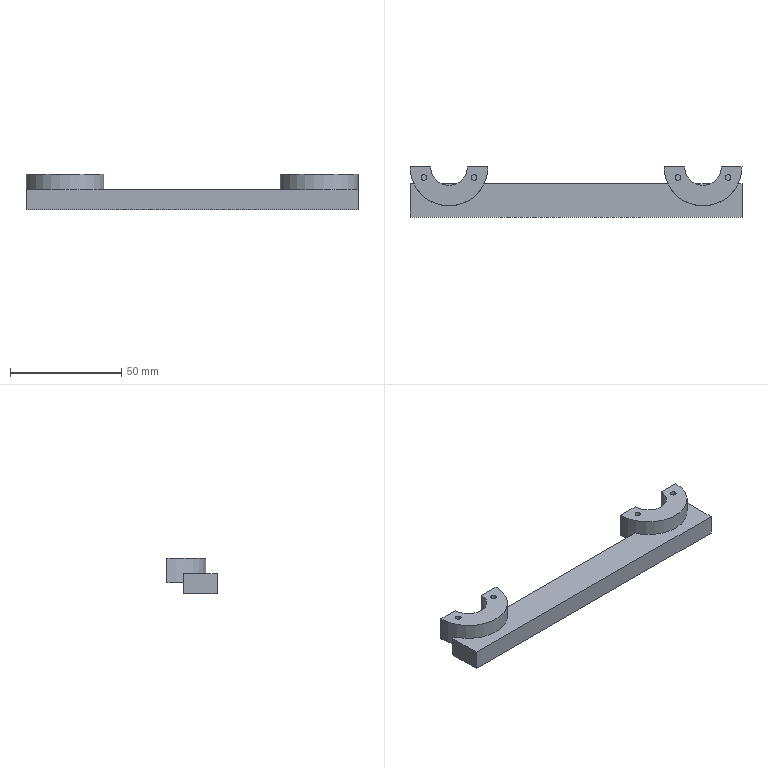NC program | NX | posted with a generic post | part box 149 x 22.5 x 16 mm
Whole program:
N10 G17 G21 G94 G90
(DRILLING , TOOL : ZXZ)
N12 T01 M6
N14 G54
N16 G17 G0 G90 X-68.25 Y4.75 S3000 M3
N18 G43 Z30. H1
N20 G94 G81 G98 Z-1. F200. R3.
N22 X-45.75
N24 X45.75
N26 X68.25
N28 G80
N30 G0 X68.25 Y4.75 Z30.
N32 M5
(DRILLING_COPY , TOOL : 2.5ZT)
N34 T02 M6
N36 G54
N38 G17 G0 G90 X-68.25 Y4.75 S200 M3
N40 G43 Z30. H2
N42 G94 G83 G98 Z-6.751 F120. Q2. R3.
N44 X-45.75
N46 X45.75
N48 X68.25
N50 G80
N52 G0 X68.25 Y4.75 Z30.
N54 M5
(DRILLING_COPY_1 , TOOL : D6A45)
N56 T03 M6
N58 G54
N60 G17 G0 G90 X-68.25 Y4.75 S3000 M3
N62 G43 Z30. H3
N64 G94 G81 G98 Z-1.4 F200. R3.
N66 X-45.75
N68 X45.75
N70 X68.25
N72 G80
N74 G0 X68.25 Y4.75 Z30.
N76 M5
N78 M2